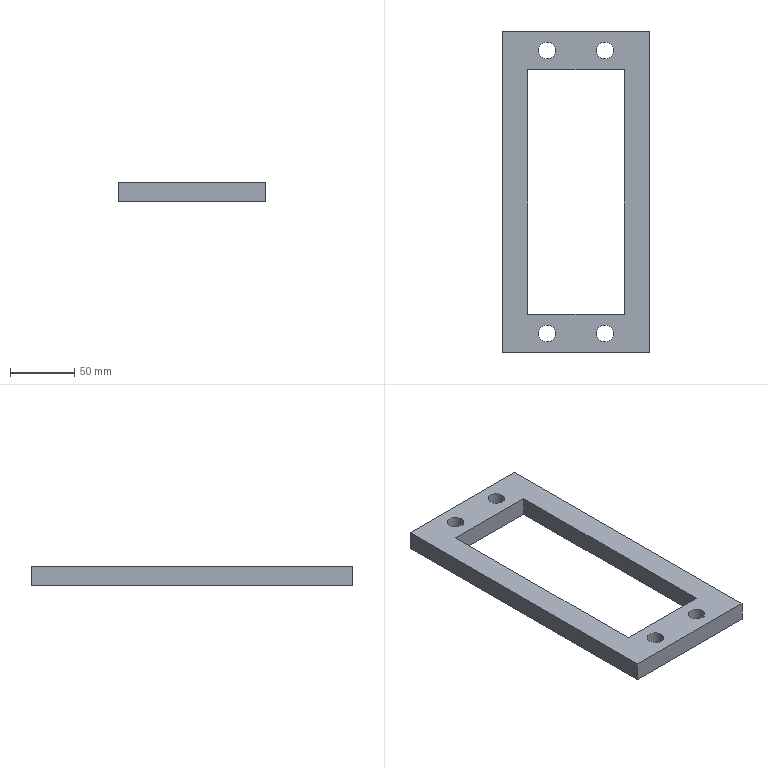Part | NX | features solid 2 | 1 solid | 14 faces | box 115 x 250 x 15 mm | volume 209536 mm3 | plane 10 | cylinder 4 | commonest cylinder face diameters 13 x4
STEP:
#1=CARTESIAN_POINT('',(447.5,30.,-85.));
#2=VERTEX_POINT('',#1);
#3=CARTESIAN_POINT('',(522.5,30.,-85.));
#4=VERTEX_POINT('',#3);
#5=CARTESIAN_POINT('',(447.5,30.,-85.));
#6=DIRECTION('',(1.,0.,0.));
#7=VECTOR('',#6,1000.);
#8=LINE('',#5,#7);
#9=EDGE_CURVE('',#2,#4,#8,.T.);
#10=ORIENTED_EDGE('',*,*,#9,.T.);
#11=CARTESIAN_POINT('',(522.5,220.,-85.));
#12=VERTEX_POINT('',#11);
#13=CARTESIAN_POINT('',(522.5,0.,-85.));
#14=DIRECTION('',(0.,1.,0.));
#15=VECTOR('',#14,1000.);
#16=LINE('',#13,#15);
#17=EDGE_CURVE('',#4,#12,#16,.T.);
#18=ORIENTED_EDGE('',*,*,#17,.T.);
#19=CARTESIAN_POINT('',(447.5,220.,-85.));
#20=VERTEX_POINT('',#19);
#21=CARTESIAN_POINT('',(522.5,220.,-85.));
#22=DIRECTION('',(-1.,0.,0.));
#23=VECTOR('',#22,1000.);
#24=LINE('',#21,#23);
#25=EDGE_CURVE('',#12,#20,#24,.T.);
#26=ORIENTED_EDGE('',*,*,#25,.T.);
#27=CARTESIAN_POINT('',(447.5,0.,-85.));
#28=DIRECTION('',(0.,1.,0.));
#29=VECTOR('',#28,1000.);
#30=LINE('',#27,#29);
#31=EDGE_CURVE('',#2,#20,#30,.T.);
#32=ORIENTED_EDGE('',*,*,#31,.F.);
#33=EDGE_LOOP('',(#10,#18,#26,#32));
#34=FACE_BOUND('',#33,.T.);
#35=CARTESIAN_POINT('',(542.5,250.,-85.));
#36=VERTEX_POINT('',#35);
#37=CARTESIAN_POINT('',(427.5,250.,-85.));
#38=VERTEX_POINT('',#37);
#39=CARTESIAN_POINT('',(522.5,250.,-85.));
#40=DIRECTION('',(-1.,0.,0.));
#41=VECTOR('',#40,1000.);
#42=LINE('',#39,#41);
#43=EDGE_CURVE('',#36,#38,#42,.T.);
#44=ORIENTED_EDGE('',*,*,#43,.F.);
#45=CARTESIAN_POINT('',(542.5,0.,-85.));
#46=VERTEX_POINT('',#45);
#47=CARTESIAN_POINT('',(542.5,0.,-85.));
#48=DIRECTION('',(0.,1.,0.));
#49=VECTOR('',#48,1000.);
#50=LINE('',#47,#49);
#51=EDGE_CURVE('',#46,#36,#50,.T.);
#52=ORIENTED_EDGE('',*,*,#51,.F.);
#53=CARTESIAN_POINT('',(427.5,0.,-85.));
#54=VERTEX_POINT('',#53);
#55=CARTESIAN_POINT('',(542.5,0.,-85.));
#56=DIRECTION('',(-1.,0.,0.));
#57=VECTOR('',#56,1000.);
#58=LINE('',#55,#57);
#59=EDGE_CURVE('',#46,#54,#58,.T.);
#60=ORIENTED_EDGE('',*,*,#59,.T.);
#61=CARTESIAN_POINT('',(427.5,0.,-85.));
#62=DIRECTION('',(0.,1.,0.));
#63=VECTOR('',#62,1000.);
#64=LINE('',#61,#63);
#65=EDGE_CURVE('',#54,#38,#64,.T.);
#66=ORIENTED_EDGE('',*,*,#65,.T.);
#67=EDGE_LOOP('',(#44,#52,#60,#66));
#68=FACE_BOUND('',#67,.T.);
#69=CARTESIAN_POINT('',(456.,235.,-85.));
#70=VERTEX_POINT('',#69);
#71=CARTESIAN_POINT('',(462.5,235.,-85.));
#72=DIRECTION('',(0.,0.,-1.));
#73=DIRECTION('',(-1.,0.,0.));
#74=AXIS2_PLACEMENT_3D('',#71,#72,#73);
#75=CIRCLE('',#74,6.5);
#76=EDGE_CURVE('',#70,#70,#75,.T.);
#77=ORIENTED_EDGE('',*,*,#76,.F.);
#78=EDGE_LOOP('',(#77));
#79=FACE_BOUND('',#78,.T.);
#80=CARTESIAN_POINT('',(501.,235.,-85.));
#81=VERTEX_POINT('',#80);
#82=CARTESIAN_POINT('',(507.5,235.,-85.));
#83=DIRECTION('',(0.,0.,-1.));
#84=DIRECTION('',(-1.,0.,0.));
#85=AXIS2_PLACEMENT_3D('',#82,#83,#84);
#86=CIRCLE('',#85,6.5);
#87=EDGE_CURVE('',#81,#81,#86,.F.);
#88=ORIENTED_EDGE('',*,*,#87,.T.);
#89=EDGE_LOOP('',(#88));
#90=FACE_BOUND('',#89,.T.);
#91=CARTESIAN_POINT('',(501.,15.,-85.));
#92=VERTEX_POINT('',#91);
#93=CARTESIAN_POINT('',(507.5,15.,-85.));
#94=DIRECTION('',(0.,0.,-1.));
#95=DIRECTION('',(-1.,0.,0.));
#96=AXIS2_PLACEMENT_3D('',#93,#94,#95);
#97=CIRCLE('',#96,6.5);
#98=EDGE_CURVE('',#92,#92,#97,.T.);
#99=ORIENTED_EDGE('',*,*,#98,.F.);
#100=EDGE_LOOP('',(#99));
#101=FACE_BOUND('',#100,.T.);
#102=CARTESIAN_POINT('',(456.,15.,-85.));
#103=VERTEX_POINT('',#102);
#104=CARTESIAN_POINT('',(462.5,15.,-85.));
#105=DIRECTION('',(0.,0.,-1.));
#106=DIRECTION('',(-1.,0.,0.));
#107=AXIS2_PLACEMENT_3D('',#104,#105,#106);
#108=CIRCLE('',#107,6.5);
#109=EDGE_CURVE('',#103,#103,#108,.F.);
#110=ORIENTED_EDGE('',*,*,#109,.T.);
#111=EDGE_LOOP('',(#110));
#112=FACE_BOUND('',#111,.T.);
#113=CARTESIAN_POINT('',(522.5,220.,-85.));
#114=DIRECTION('',(0.,0.,-1.));
#115=DIRECTION('',(-1.,0.,0.));
#116=AXIS2_PLACEMENT_3D('',#113,#114,#115);
#117=PLANE('',#116);
#118=ADVANCED_FACE('',(#34,#68,#79,#90,#101,#112),#117,.T.);
#119=CARTESIAN_POINT('',(522.5,30.,-70.));
#120=VERTEX_POINT('',#119);
#121=CARTESIAN_POINT('',(522.5,220.,-70.));
#122=VERTEX_POINT('',#121);
#123=CARTESIAN_POINT('',(522.5,0.,-70.));
#124=DIRECTION('',(0.,1.,0.));
#125=VECTOR('',#124,1000.);
#126=LINE('',#123,#125);
#127=EDGE_CURVE('',#120,#122,#126,.T.);
#128=ORIENTED_EDGE('',*,*,#127,.F.);
#129=CARTESIAN_POINT('',(447.5,30.,-70.));
#130=VERTEX_POINT('',#129);
#131=CARTESIAN_POINT('',(447.5,30.,-70.));
#132=DIRECTION('',(-1.,0.,0.));
#133=VECTOR('',#132,1000.);
#134=LINE('',#131,#133);
#135=EDGE_CURVE('',#130,#120,#134,.F.);
#136=ORIENTED_EDGE('',*,*,#135,.F.);
#137=CARTESIAN_POINT('',(447.5,220.,-70.));
#138=VERTEX_POINT('',#137);
#139=CARTESIAN_POINT('',(447.5,0.,-70.));
#140=DIRECTION('',(0.,1.,0.));
#141=VECTOR('',#140,1000.);
#142=LINE('',#139,#141);
#143=EDGE_CURVE('',#130,#138,#142,.T.);
#144=ORIENTED_EDGE('',*,*,#143,.T.);
#145=CARTESIAN_POINT('',(522.5,220.,-70.));
#146=DIRECTION('',(-1.,0.,0.));
#147=VECTOR('',#146,1000.);
#148=LINE('',#145,#147);
#149=EDGE_CURVE('',#122,#138,#148,.T.);
#150=ORIENTED_EDGE('',*,*,#149,.F.);
#151=EDGE_LOOP('',(#128,#136,#144,#150));
#152=FACE_BOUND('',#151,.T.);
#153=CARTESIAN_POINT('',(542.5,250.,-70.));
#154=VERTEX_POINT('',#153);
#155=CARTESIAN_POINT('',(427.5,250.,-70.));
#156=VERTEX_POINT('',#155);
#157=CARTESIAN_POINT('',(522.5,250.,-70.));
#158=DIRECTION('',(-1.,0.,0.));
#159=VECTOR('',#158,1000.);
#160=LINE('',#157,#159);
#161=EDGE_CURVE('',#154,#156,#160,.T.);
#162=ORIENTED_EDGE('',*,*,#161,.T.);
#163=CARTESIAN_POINT('',(427.5,0.,-70.));
#164=VERTEX_POINT('',#163);
#165=CARTESIAN_POINT('',(427.5,0.,-70.));
#166=DIRECTION('',(0.,1.,0.));
#167=VECTOR('',#166,1000.);
#168=LINE('',#165,#167);
#169=EDGE_CURVE('',#164,#156,#168,.T.);
#170=ORIENTED_EDGE('',*,*,#169,.F.);
#171=CARTESIAN_POINT('',(542.5,0.,-70.));
#172=VERTEX_POINT('',#171);
#173=CARTESIAN_POINT('',(542.5,0.,-70.));
#174=DIRECTION('',(-1.,0.,0.));
#175=VECTOR('',#174,1000.);
#176=LINE('',#173,#175);
#177=EDGE_CURVE('',#172,#164,#176,.T.);
#178=ORIENTED_EDGE('',*,*,#177,.F.);
#179=CARTESIAN_POINT('',(542.5,0.,-70.));
#180=DIRECTION('',(0.,1.,0.));
#181=VECTOR('',#180,1000.);
#182=LINE('',#179,#181);
#183=EDGE_CURVE('',#172,#154,#182,.T.);
#184=ORIENTED_EDGE('',*,*,#183,.T.);
#185=EDGE_LOOP('',(#162,#170,#178,#184));
#186=FACE_BOUND('',#185,.T.);
#187=CARTESIAN_POINT('',(456.,235.,-70.));
#188=VERTEX_POINT('',#187);
#189=CARTESIAN_POINT('',(462.5,235.,-70.));
#190=DIRECTION('',(0.,0.,-1.));
#191=DIRECTION('',(-1.,0.,0.));
#192=AXIS2_PLACEMENT_3D('',#189,#190,#191);
#193=CIRCLE('',#192,6.5);
#194=EDGE_CURVE('',#188,#188,#193,.T.);
#195=ORIENTED_EDGE('',*,*,#194,.T.);
#196=EDGE_LOOP('',(#195));
#197=FACE_BOUND('',#196,.T.);
#198=CARTESIAN_POINT('',(501.,235.,-70.));
#199=VERTEX_POINT('',#198);
#200=CARTESIAN_POINT('',(507.5,235.,-70.));
#201=DIRECTION('',(0.,0.,-1.));
#202=DIRECTION('',(-1.,0.,0.));
#203=AXIS2_PLACEMENT_3D('',#200,#201,#202);
#204=CIRCLE('',#203,6.5);
#205=EDGE_CURVE('',#199,#199,#204,.F.);
#206=ORIENTED_EDGE('',*,*,#205,.F.);
#207=EDGE_LOOP('',(#206));
#208=FACE_BOUND('',#207,.T.);
#209=CARTESIAN_POINT('',(501.,15.,-70.));
#210=VERTEX_POINT('',#209);
#211=CARTESIAN_POINT('',(507.5,15.,-70.));
#212=DIRECTION('',(0.,0.,-1.));
#213=DIRECTION('',(-1.,0.,0.));
#214=AXIS2_PLACEMENT_3D('',#211,#212,#213);
#215=CIRCLE('',#214,6.5);
#216=EDGE_CURVE('',#210,#210,#215,.T.);
#217=ORIENTED_EDGE('',*,*,#216,.T.);
#218=EDGE_LOOP('',(#217));
#219=FACE_BOUND('',#218,.T.);
#220=CARTESIAN_POINT('',(456.,15.,-70.));
#221=VERTEX_POINT('',#220);
#222=CARTESIAN_POINT('',(462.5,15.,-70.));
#223=DIRECTION('',(0.,0.,-1.));
#224=DIRECTION('',(-1.,0.,0.));
#225=AXIS2_PLACEMENT_3D('',#222,#223,#224);
#226=CIRCLE('',#225,6.5);
#227=EDGE_CURVE('',#221,#221,#226,.F.);
#228=ORIENTED_EDGE('',*,*,#227,.F.);
#229=EDGE_LOOP('',(#228));
#230=FACE_BOUND('',#229,.T.);
#231=CARTESIAN_POINT('',(522.5,220.,-70.));
#232=DIRECTION('',(0.,0.,-1.));
#233=DIRECTION('',(-1.,0.,0.));
#234=AXIS2_PLACEMENT_3D('',#231,#232,#233);
#235=PLANE('',#234);
#236=ADVANCED_FACE('',(#152,#186,#197,#208,#219,#230),#235,.F.);
#237=CARTESIAN_POINT('',(522.5,220.,-85.));
#238=DIRECTION('',(0.,0.,-1.));
#239=VECTOR('',#238,1000.);
#240=LINE('',#237,#239);
#241=EDGE_CURVE('',#12,#122,#240,.F.);
#242=ORIENTED_EDGE('',*,*,#241,.T.);
#243=ORIENTED_EDGE('',*,*,#149,.T.);
#244=CARTESIAN_POINT('',(447.5,220.,-85.));
#245=DIRECTION('',(0.,0.,-1.));
#246=VECTOR('',#245,1000.);
#247=LINE('',#244,#246);
#248=EDGE_CURVE('',#20,#138,#247,.F.);
#249=ORIENTED_EDGE('',*,*,#248,.F.);
#250=ORIENTED_EDGE('',*,*,#25,.F.);
#251=EDGE_LOOP('',(#242,#243,#249,#250));
#252=FACE_BOUND('',#251,.T.);
#253=CARTESIAN_POINT('',(522.5,220.,-85.));
#254=DIRECTION('',(0.,-1.,0.));
#255=DIRECTION('',(-1.,0.,0.));
#256=AXIS2_PLACEMENT_3D('',#253,#254,#255);
#257=PLANE('',#256);
#258=ADVANCED_FACE('',(#252),#257,.T.);
#259=ORIENTED_EDGE('',*,*,#43,.T.);
#260=CARTESIAN_POINT('',(427.5,250.,-85.));
#261=DIRECTION('',(0.,0.,-1.));
#262=VECTOR('',#261,1000.);
#263=LINE('',#260,#262);
#264=EDGE_CURVE('',#38,#156,#263,.F.);
#265=ORIENTED_EDGE('',*,*,#264,.T.);
#266=ORIENTED_EDGE('',*,*,#161,.F.);
#267=CARTESIAN_POINT('',(542.5,250.,-85.));
#268=DIRECTION('',(0.,0.,1.));
#269=VECTOR('',#268,1000.);
#270=LINE('',#267,#269);
#271=EDGE_CURVE('',#36,#154,#270,.T.);
#272=ORIENTED_EDGE('',*,*,#271,.F.);
#273=EDGE_LOOP('',(#259,#265,#266,#272));
#274=FACE_BOUND('',#273,.T.);
#275=CARTESIAN_POINT('',(522.5,250.,-85.));
#276=DIRECTION('',(0.,-1.,0.));
#277=DIRECTION('',(-1.,0.,0.));
#278=AXIS2_PLACEMENT_3D('',#275,#276,#277);
#279=PLANE('',#278);
#280=ADVANCED_FACE('',(#274),#279,.F.);
#281=ORIENTED_EDGE('',*,*,#76,.T.);
#282=EDGE_LOOP('',(#281));
#283=FACE_BOUND('',#282,.T.);
#284=ORIENTED_EDGE('',*,*,#194,.F.);
#285=EDGE_LOOP('',(#284));
#286=FACE_BOUND('',#285,.T.);
#287=CARTESIAN_POINT('',(462.5,235.,-95.));
#288=DIRECTION('',(0.,0.,1.));
#289=DIRECTION('',(1.,0.,0.));
#290=AXIS2_PLACEMENT_3D('',#287,#288,#289);
#291=CYLINDRICAL_SURFACE('',#290,6.5);
#292=ADVANCED_FACE('',(#283,#286),#291,.F.);
#293=ORIENTED_EDGE('',*,*,#87,.F.);
#294=EDGE_LOOP('',(#293));
#295=FACE_BOUND('',#294,.T.);
#296=ORIENTED_EDGE('',*,*,#205,.T.);
#297=EDGE_LOOP('',(#296));
#298=FACE_BOUND('',#297,.T.);
#299=CARTESIAN_POINT('',(507.5,235.,-84.));
#300=DIRECTION('',(0.,0.,1.));
#301=DIRECTION('',(1.,0.,0.));
#302=AXIS2_PLACEMENT_3D('',#299,#300,#301);
#303=CYLINDRICAL_SURFACE('',#302,6.5);
#304=ADVANCED_FACE('',(#295,#298),#303,.F.);
#305=CARTESIAN_POINT('',(522.5,30.,-85.));
#306=DIRECTION('',(0.,0.,1.));
#307=VECTOR('',#306,1000.);
#308=LINE('',#305,#307);
#309=EDGE_CURVE('',#4,#120,#308,.T.);
#310=ORIENTED_EDGE('',*,*,#309,.T.);
#311=ORIENTED_EDGE('',*,*,#127,.T.);
#312=ORIENTED_EDGE('',*,*,#241,.F.);
#313=ORIENTED_EDGE('',*,*,#17,.F.);
#314=EDGE_LOOP('',(#310,#311,#312,#313));
#315=FACE_BOUND('',#314,.T.);
#316=CARTESIAN_POINT('',(522.5,0.,-85.));
#317=DIRECTION('',(1.,0.,0.));
#318=DIRECTION('',(0.,0.,1.));
#319=AXIS2_PLACEMENT_3D('',#316,#317,#318);
#320=PLANE('',#319);
#321=ADVANCED_FACE('',(#315),#320,.F.);
#322=ORIENTED_EDGE('',*,*,#183,.F.);
#323=CARTESIAN_POINT('',(542.5,0.,-85.));
#324=DIRECTION('',(0.,0.,1.));
#325=VECTOR('',#324,1000.);
#326=LINE('',#323,#325);
#327=EDGE_CURVE('',#46,#172,#326,.T.);
#328=ORIENTED_EDGE('',*,*,#327,.F.);
#329=ORIENTED_EDGE('',*,*,#51,.T.);
#330=ORIENTED_EDGE('',*,*,#271,.T.);
#331=EDGE_LOOP('',(#322,#328,#329,#330));
#332=FACE_BOUND('',#331,.T.);
#333=CARTESIAN_POINT('',(542.5,0.,-85.));
#334=DIRECTION('',(1.,0.,0.));
#335=DIRECTION('',(0.,0.,1.));
#336=AXIS2_PLACEMENT_3D('',#333,#334,#335);
#337=PLANE('',#336);
#338=ADVANCED_FACE('',(#332),#337,.T.);
#339=ORIENTED_EDGE('',*,*,#177,.T.);
#340=CARTESIAN_POINT('',(427.5,0.,-85.));
#341=DIRECTION('',(0.,0.,1.));
#342=VECTOR('',#341,1000.);
#343=LINE('',#340,#342);
#344=EDGE_CURVE('',#54,#164,#343,.T.);
#345=ORIENTED_EDGE('',*,*,#344,.F.);
#346=ORIENTED_EDGE('',*,*,#59,.F.);
#347=ORIENTED_EDGE('',*,*,#327,.T.);
#348=EDGE_LOOP('',(#339,#345,#346,#347));
#349=FACE_BOUND('',#348,.T.);
#350=CARTESIAN_POINT('',(542.5,0.,-85.));
#351=DIRECTION('',(0.,-1.,0.));
#352=DIRECTION('',(0.,0.,-1.));
#353=AXIS2_PLACEMENT_3D('',#350,#351,#352);
#354=PLANE('',#353);
#355=ADVANCED_FACE('',(#349),#354,.T.);
#356=ORIENTED_EDGE('',*,*,#65,.F.);
#357=ORIENTED_EDGE('',*,*,#344,.T.);
#358=ORIENTED_EDGE('',*,*,#169,.T.);
#359=ORIENTED_EDGE('',*,*,#264,.F.);
#360=EDGE_LOOP('',(#356,#357,#358,#359));
#361=FACE_BOUND('',#360,.T.);
#362=CARTESIAN_POINT('',(427.5,0.,-85.));
#363=DIRECTION('',(-1.,0.,0.));
#364=DIRECTION('',(0.,0.,1.));
#365=AXIS2_PLACEMENT_3D('',#362,#363,#364);
#366=PLANE('',#365);
#367=ADVANCED_FACE('',(#361),#366,.T.);
#368=CARTESIAN_POINT('',(447.5,30.,-85.));
#369=DIRECTION('',(0.,0.,1.));
#370=VECTOR('',#369,1000.);
#371=LINE('',#368,#370);
#372=EDGE_CURVE('',#2,#130,#371,.T.);
#373=ORIENTED_EDGE('',*,*,#372,.F.);
#374=ORIENTED_EDGE('',*,*,#31,.T.);
#375=ORIENTED_EDGE('',*,*,#248,.T.);
#376=ORIENTED_EDGE('',*,*,#143,.F.);
#377=EDGE_LOOP('',(#373,#374,#375,#376));
#378=FACE_BOUND('',#377,.T.);
#379=CARTESIAN_POINT('',(447.5,0.,-85.));
#380=DIRECTION('',(-1.,0.,0.));
#381=DIRECTION('',(0.,0.,1.));
#382=AXIS2_PLACEMENT_3D('',#379,#380,#381);
#383=PLANE('',#382);
#384=ADVANCED_FACE('',(#378),#383,.F.);
#385=ORIENTED_EDGE('',*,*,#309,.F.);
#386=ORIENTED_EDGE('',*,*,#9,.F.);
#387=ORIENTED_EDGE('',*,*,#372,.T.);
#388=ORIENTED_EDGE('',*,*,#135,.T.);
#389=EDGE_LOOP('',(#385,#386,#387,#388));
#390=FACE_BOUND('',#389,.T.);
#391=CARTESIAN_POINT('',(447.5,30.,-85.));
#392=DIRECTION('',(0.,1.,0.));
#393=DIRECTION('',(1.,0.,0.));
#394=AXIS2_PLACEMENT_3D('',#391,#392,#393);
#395=PLANE('',#394);
#396=ADVANCED_FACE('',(#390),#395,.T.);
#397=ORIENTED_EDGE('',*,*,#109,.F.);
#398=EDGE_LOOP('',(#397));
#399=FACE_BOUND('',#398,.T.);
#400=ORIENTED_EDGE('',*,*,#227,.T.);
#401=EDGE_LOOP('',(#400));
#402=FACE_BOUND('',#401,.T.);
#403=CARTESIAN_POINT('',(462.5,15.,-95.));
#404=DIRECTION('',(0.,0.,1.));
#405=DIRECTION('',(1.,0.,0.));
#406=AXIS2_PLACEMENT_3D('',#403,#404,#405);
#407=CYLINDRICAL_SURFACE('',#406,6.5);
#408=ADVANCED_FACE('',(#399,#402),#407,.F.);
#409=ORIENTED_EDGE('',*,*,#98,.T.);
#410=EDGE_LOOP('',(#409));
#411=FACE_BOUND('',#410,.T.);
#412=ORIENTED_EDGE('',*,*,#216,.F.);
#413=EDGE_LOOP('',(#412));
#414=FACE_BOUND('',#413,.T.);
#415=CARTESIAN_POINT('',(507.5,15.,-95.));
#416=DIRECTION('',(0.,0.,1.));
#417=DIRECTION('',(1.,0.,0.));
#418=AXIS2_PLACEMENT_3D('',#415,#416,#417);
#419=CYLINDRICAL_SURFACE('',#418,6.5);
#420=ADVANCED_FACE('',(#411,#414),#419,.F.);
#421=CLOSED_SHELL('',(#118,#236,#258,#280,#292,#304,#321,#338,#355,#367,#384,#396,#408,#420));
#422=MANIFOLD_SOLID_BREP('',#421);
#423=(LENGTH_UNIT()NAMED_UNIT(*)SI_UNIT(.MILLI.,.METRE.));
#424=UNCERTAINTY_MEASURE_WITH_UNIT(LENGTH_MEASURE(0.00001),#423,'','');
#425=(NAMED_UNIT(*)PLANE_ANGLE_UNIT()SI_UNIT($,.RADIAN.));
#426=(NAMED_UNIT(*)SI_UNIT($,.STERADIAN.)SOLID_ANGLE_UNIT());
#427=(GEOMETRIC_REPRESENTATION_CONTEXT(3)GLOBAL_UNCERTAINTY_ASSIGNED_CONTEXT((#424))GLOBAL_UNIT_ASSIGNED_CONTEXT((#423,#425,#426))REPRESENTATION_CONTEXT('',''));
#428=ADVANCED_BREP_SHAPE_REPRESENTATION('',(#422),#427);